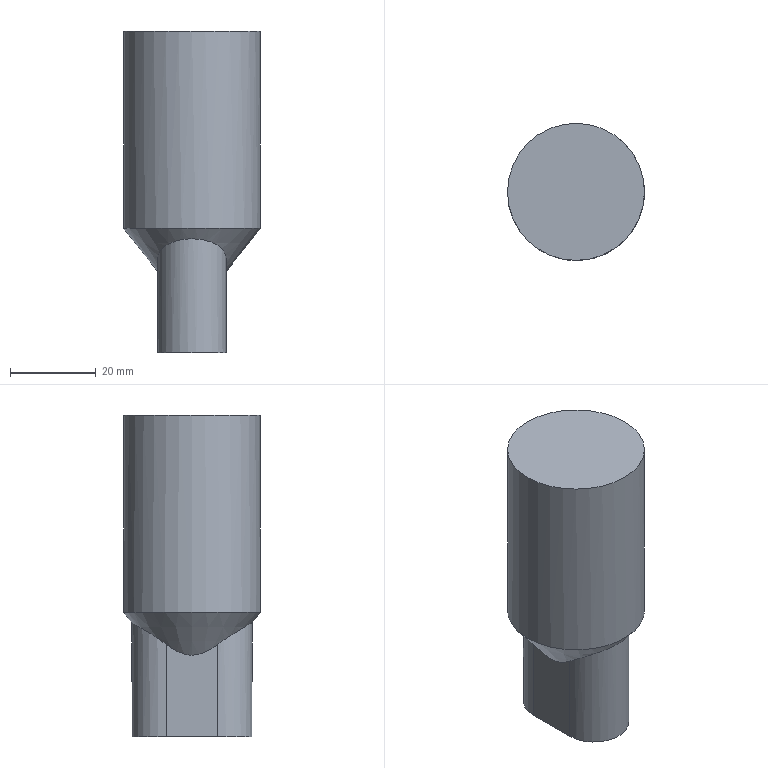Part | NX | features solid 2 | 1 solid | 8 faces | box 32 x 32 x 75 mm | volume 49860 mm3 | plane 4 | cylinder 3 | cone 1 | commonest cylinder face diameters 16.1 x2 32 x1
STEP:
#1=CARTESIAN_POINT('',(-404.123,-158.946,54.503));
#2=VERTEX_POINT('',#1);
#3=CARTESIAN_POINT('',(-404.128,-146.946,54.503));
#4=VERTEX_POINT('',#3);
#5=CARTESIAN_POINT('',(-404.123,-158.946,54.503));
#6=CARTESIAN_POINT('',(-404.123,-158.063,53.839));
#7=CARTESIAN_POINT('',(-404.124,-156.235,52.619));
#8=CARTESIAN_POINT('',(-404.125,-152.94,51.691));
#9=CARTESIAN_POINT('',(-404.126,-149.667,52.616));
#10=CARTESIAN_POINT('',(-404.127,-147.831,53.838));
#11=CARTESIAN_POINT('',(-404.128,-146.946,54.503));
#12=B_SPLINE_CURVE_WITH_KNOTS('',3,(#5,#6,#7,#8,#9,#10,#11),.UNSPECIFIED.,.F.,.F.,(4,1,1,1,4),(0.000000249,0.003296,0.006591,0.009886,0.01318),.UNSPECIFIED.);
#13=EDGE_CURVE('',#2,#4,#12,.T.);
#14=ORIENTED_EDGE('',*,*,#13,.F.);
#15=CARTESIAN_POINT('',(-404.123,-158.946,33.));
#16=VERTEX_POINT('',#15);
#17=CARTESIAN_POINT('',(-404.123,-158.946,33.));
#18=DIRECTION('',(0.,0.,1.));
#19=VECTOR('',#18,1000.);
#20=LINE('',#17,#19);
#21=EDGE_CURVE('',#16,#2,#20,.T.);
#22=ORIENTED_EDGE('',*,*,#21,.F.);
#23=CARTESIAN_POINT('',(-404.128,-146.946,33.));
#24=VERTEX_POINT('',#23);
#25=CARTESIAN_POINT('',(-404.125,-152.946,33.));
#26=DIRECTION('',(-0.000407,1.,0.));
#27=VECTOR('',#26,1000.);
#28=LINE('',#25,#27);
#29=EDGE_CURVE('',#16,#24,#28,.T.);
#30=ORIENTED_EDGE('',*,*,#29,.T.);
#31=CARTESIAN_POINT('',(-404.128,-146.946,33.));
#32=DIRECTION('',(0.,0.,1.));
#33=VECTOR('',#32,1000.);
#34=LINE('',#31,#33);
#35=EDGE_CURVE('',#24,#4,#34,.T.);
#36=ORIENTED_EDGE('',*,*,#35,.T.);
#37=EDGE_LOOP('',(#14,#22,#30,#36));
#38=FACE_BOUND('',#37,.T.);
#39=CARTESIAN_POINT('',(-404.125,-152.946,33.));
#40=DIRECTION('',(1.,0.000407,0.));
#41=DIRECTION('',(0.,0.,1.));
#42=AXIS2_PLACEMENT_3D('',#39,#40,#41);
#43=PLANE('',#42);
#44=ADVANCED_FACE('',(#38),#43,.T.);
#45=ORIENTED_EDGE('',*,*,#29,.F.);
#46=CARTESIAN_POINT('',(-420.223,-158.953,33.));
#47=VERTEX_POINT('',#46);
#48=CARTESIAN_POINT('',(-412.173,-158.95,33.));
#49=DIRECTION('',(0.,0.,1.));
#50=DIRECTION('',(-1.,-0.000407,0.));
#51=AXIS2_PLACEMENT_3D('',#48,#49,#50);
#52=CIRCLE('',#51,8.05);
#53=EDGE_CURVE('',#47,#16,#52,.T.);
#54=ORIENTED_EDGE('',*,*,#53,.F.);
#55=CARTESIAN_POINT('',(-420.228,-146.953,33.));
#56=VERTEX_POINT('',#55);
#57=CARTESIAN_POINT('',(-420.225,-152.953,33.));
#58=DIRECTION('',(0.000407,-1.,0.));
#59=VECTOR('',#58,1000.);
#60=LINE('',#57,#59);
#61=EDGE_CURVE('',#56,#47,#60,.T.);
#62=ORIENTED_EDGE('',*,*,#61,.F.);
#63=CARTESIAN_POINT('',(-412.178,-146.95,33.));
#64=DIRECTION('',(0.,0.,1.));
#65=DIRECTION('',(-1.,-0.000407,0.));
#66=AXIS2_PLACEMENT_3D('',#63,#64,#65);
#67=CIRCLE('',#66,8.05);
#68=EDGE_CURVE('',#24,#56,#67,.T.);
#69=ORIENTED_EDGE('',*,*,#68,.F.);
#70=EDGE_LOOP('',(#45,#54,#62,#69));
#71=FACE_BOUND('',#70,.T.);
#72=CARTESIAN_POINT('',(-412.175,-152.95,33.));
#73=DIRECTION('',(0.,0.,-1.));
#74=DIRECTION('',(1.,0.000407,0.));
#75=AXIS2_PLACEMENT_3D('',#72,#73,#74);
#76=PLANE('',#75);
#77=ADVANCED_FACE('',(#71),#76,.T.);
#78=CARTESIAN_POINT('',(-420.228,-146.953,54.503));
#79=VERTEX_POINT('',#78);
#80=CARTESIAN_POINT('',(-420.223,-158.953,54.503));
#81=VERTEX_POINT('',#80);
#82=CARTESIAN_POINT('',(-420.228,-146.953,54.503));
#83=CARTESIAN_POINT('',(-420.227,-147.837,53.839));
#84=CARTESIAN_POINT('',(-420.226,-149.664,52.619));
#85=CARTESIAN_POINT('',(-420.225,-152.959,51.691));
#86=CARTESIAN_POINT('',(-420.224,-156.232,52.616));
#87=CARTESIAN_POINT('',(-420.223,-158.069,53.838));
#88=CARTESIAN_POINT('',(-420.223,-158.953,54.503));
#89=B_SPLINE_CURVE_WITH_KNOTS('',3,(#82,#83,#84,#85,#86,#87,#88),.UNSPECIFIED.,.F.,.F.,(4,1,1,1,4),(0.000000249,0.003296,0.006591,0.009886,0.01318),.UNSPECIFIED.);
#90=EDGE_CURVE('',#79,#81,#89,.T.);
#91=ORIENTED_EDGE('',*,*,#90,.F.);
#92=CARTESIAN_POINT('',(-420.228,-146.953,33.));
#93=DIRECTION('',(0.,0.,1.));
#94=VECTOR('',#93,1000.);
#95=LINE('',#92,#94);
#96=EDGE_CURVE('',#56,#79,#95,.T.);
#97=ORIENTED_EDGE('',*,*,#96,.F.);
#98=ORIENTED_EDGE('',*,*,#61,.T.);
#99=CARTESIAN_POINT('',(-420.223,-158.953,33.));
#100=DIRECTION('',(0.,0.,1.));
#101=VECTOR('',#100,1000.);
#102=LINE('',#99,#101);
#103=EDGE_CURVE('',#47,#81,#102,.T.);
#104=ORIENTED_EDGE('',*,*,#103,.T.);
#105=EDGE_LOOP('',(#91,#97,#98,#104));
#106=FACE_BOUND('',#105,.T.);
#107=CARTESIAN_POINT('',(-420.225,-152.953,33.));
#108=DIRECTION('',(-1.,-0.000407,0.));
#109=DIRECTION('',(0.,0.,-1.));
#110=AXIS2_PLACEMENT_3D('',#107,#108,#109);
#111=PLANE('',#110);
#112=ADVANCED_FACE('',(#106),#111,.T.);
#113=CARTESIAN_POINT('',(-404.123,-158.946,54.503));
#114=CARTESIAN_POINT('',(-404.122,-160.79,55.889));
#115=CARTESIAN_POINT('',(-405.112,-163.763,57.76));
#116=CARTESIAN_POINT('',(-408.673,-166.468,59.265));
#117=CARTESIAN_POINT('',(-412.138,-167.257,59.684));
#118=CARTESIAN_POINT('',(-415.606,-166.5,59.281));
#119=CARTESIAN_POINT('',(-419.219,-163.802,57.78));
#120=CARTESIAN_POINT('',(-420.222,-160.799,55.891));
#121=CARTESIAN_POINT('',(-420.223,-158.953,54.503));
#122=B_SPLINE_CURVE_WITH_KNOTS('',3,(#113,#114,#115,#116,#117,#118,#119,#120,#121),.UNSPECIFIED.,.F.,.F.,(4,1,1,1,1,1,4),(0.003949,0.01081,0.01424,0.01767,0.02109,0.02452,0.03138),.UNSPECIFIED.);
#123=EDGE_CURVE('',#2,#81,#122,.T.);
#124=ORIENTED_EDGE('',*,*,#123,.F.);
#125=ORIENTED_EDGE('',*,*,#13,.T.);
#126=CARTESIAN_POINT('',(-420.228,-146.953,54.503));
#127=CARTESIAN_POINT('',(-420.228,-145.109,55.889));
#128=CARTESIAN_POINT('',(-419.238,-142.136,57.76));
#129=CARTESIAN_POINT('',(-415.677,-139.431,59.265));
#130=CARTESIAN_POINT('',(-412.212,-138.642,59.684));
#131=CARTESIAN_POINT('',(-408.744,-139.399,59.281));
#132=CARTESIAN_POINT('',(-405.131,-142.097,57.78));
#133=CARTESIAN_POINT('',(-404.128,-145.1,55.891));
#134=CARTESIAN_POINT('',(-404.128,-146.946,54.503));
#135=B_SPLINE_CURVE_WITH_KNOTS('',3,(#126,#127,#128,#129,#130,#131,#132,#133,#134),.UNSPECIFIED.,.F.,.F.,(4,1,1,1,1,1,4),(0.003949,0.01081,0.01424,0.01767,0.02109,0.02452,0.03138),.UNSPECIFIED.);
#136=EDGE_CURVE('',#79,#4,#135,.T.);
#137=ORIENTED_EDGE('',*,*,#136,.F.);
#138=ORIENTED_EDGE('',*,*,#90,.T.);
#139=EDGE_LOOP('',(#124,#125,#137,#138));
#140=FACE_BOUND('',#139,.T.);
#141=CARTESIAN_POINT('',(-428.175,-152.956,62.));
#142=VERTEX_POINT('',#141);
#143=CARTESIAN_POINT('',(-412.175,-152.95,62.));
#144=DIRECTION('',(0.,0.,1.));
#145=DIRECTION('',(-1.,-0.000407,0.));
#146=AXIS2_PLACEMENT_3D('',#143,#144,#145);
#147=CIRCLE('',#146,16.);
#148=EDGE_CURVE('',#142,#142,#147,.T.);
#149=ORIENTED_EDGE('',*,*,#148,.F.);
#150=EDGE_LOOP('',(#149));
#151=FACE_BOUND('',#150,.T.);
#152=CARTESIAN_POINT('',(-412.175,-152.95,52.));
#153=DIRECTION('',(0.,0.,1.));
#154=DIRECTION('',(-1.,-0.000407,0.));
#155=AXIS2_PLACEMENT_3D('',#152,#153,#154);
#156=CONICAL_SURFACE('',#155,8.05,0.6717);
#157=ADVANCED_FACE('',(#140,#151),#156,.T.);
#158=CARTESIAN_POINT('',(-396.175,-152.943,108.));
#159=VERTEX_POINT('',#158);
#160=CARTESIAN_POINT('',(-412.175,-152.95,108.));
#161=DIRECTION('',(0.,0.,-1.));
#162=DIRECTION('',(1.,0.000407,0.));
#163=AXIS2_PLACEMENT_3D('',#160,#161,#162);
#164=CIRCLE('',#163,16.);
#165=EDGE_CURVE('',#159,#159,#164,.T.);
#166=ORIENTED_EDGE('',*,*,#165,.F.);
#167=EDGE_LOOP('',(#166));
#168=FACE_BOUND('',#167,.T.);
#169=CARTESIAN_POINT('',(-412.175,-152.95,108.));
#170=DIRECTION('',(0.,0.,1.));
#171=DIRECTION('',(-1.,-0.000407,0.));
#172=AXIS2_PLACEMENT_3D('',#169,#170,#171);
#173=PLANE('',#172);
#174=ADVANCED_FACE('',(#168),#173,.T.);
#175=ORIENTED_EDGE('',*,*,#165,.T.);
#176=EDGE_LOOP('',(#175));
#177=FACE_BOUND('',#176,.T.);
#178=ORIENTED_EDGE('',*,*,#148,.T.);
#179=EDGE_LOOP('',(#178));
#180=FACE_BOUND('',#179,.T.);
#181=CARTESIAN_POINT('',(-412.175,-152.95,62.));
#182=DIRECTION('',(0.,0.,1.));
#183=DIRECTION('',(-1.,-0.000407,0.));
#184=AXIS2_PLACEMENT_3D('',#181,#182,#183);
#185=CYLINDRICAL_SURFACE('',#184,16.);
#186=ADVANCED_FACE('',(#177,#180),#185,.T.);
#187=ORIENTED_EDGE('',*,*,#35,.F.);
#188=ORIENTED_EDGE('',*,*,#68,.T.);
#189=ORIENTED_EDGE('',*,*,#96,.T.);
#190=ORIENTED_EDGE('',*,*,#136,.T.);
#191=EDGE_LOOP('',(#187,#188,#189,#190));
#192=FACE_BOUND('',#191,.T.);
#193=CARTESIAN_POINT('',(-412.178,-146.95,33.));
#194=DIRECTION('',(0.,0.,1.));
#195=DIRECTION('',(-1.,-0.000407,0.));
#196=AXIS2_PLACEMENT_3D('',#193,#194,#195);
#197=CYLINDRICAL_SURFACE('',#196,8.05);
#198=ADVANCED_FACE('',(#192),#197,.T.);
#199=ORIENTED_EDGE('',*,*,#53,.T.);
#200=ORIENTED_EDGE('',*,*,#21,.T.);
#201=ORIENTED_EDGE('',*,*,#123,.T.);
#202=ORIENTED_EDGE('',*,*,#103,.F.);
#203=EDGE_LOOP('',(#199,#200,#201,#202));
#204=FACE_BOUND('',#203,.T.);
#205=CARTESIAN_POINT('',(-412.173,-158.95,33.));
#206=DIRECTION('',(0.,0.,1.));
#207=DIRECTION('',(-1.,-0.000407,0.));
#208=AXIS2_PLACEMENT_3D('',#205,#206,#207);
#209=CYLINDRICAL_SURFACE('',#208,8.05);
#210=ADVANCED_FACE('',(#204),#209,.T.);
#211=CLOSED_SHELL('',(#44,#77,#112,#157,#174,#186,#198,#210));
#212=MANIFOLD_SOLID_BREP('',#211);
#213=(LENGTH_UNIT()NAMED_UNIT(*)SI_UNIT(.MILLI.,.METRE.));
#214=UNCERTAINTY_MEASURE_WITH_UNIT(LENGTH_MEASURE(0.0508),#213,'','');
#215=(NAMED_UNIT(*)PLANE_ANGLE_UNIT()SI_UNIT($,.RADIAN.));
#216=(NAMED_UNIT(*)SI_UNIT($,.STERADIAN.)SOLID_ANGLE_UNIT());
#217=(GEOMETRIC_REPRESENTATION_CONTEXT(3)GLOBAL_UNCERTAINTY_ASSIGNED_CONTEXT((#214))GLOBAL_UNIT_ASSIGNED_CONTEXT((#213,#215,#216))REPRESENTATION_CONTEXT('',''));
#218=ADVANCED_BREP_SHAPE_REPRESENTATION('',(#212),#217);